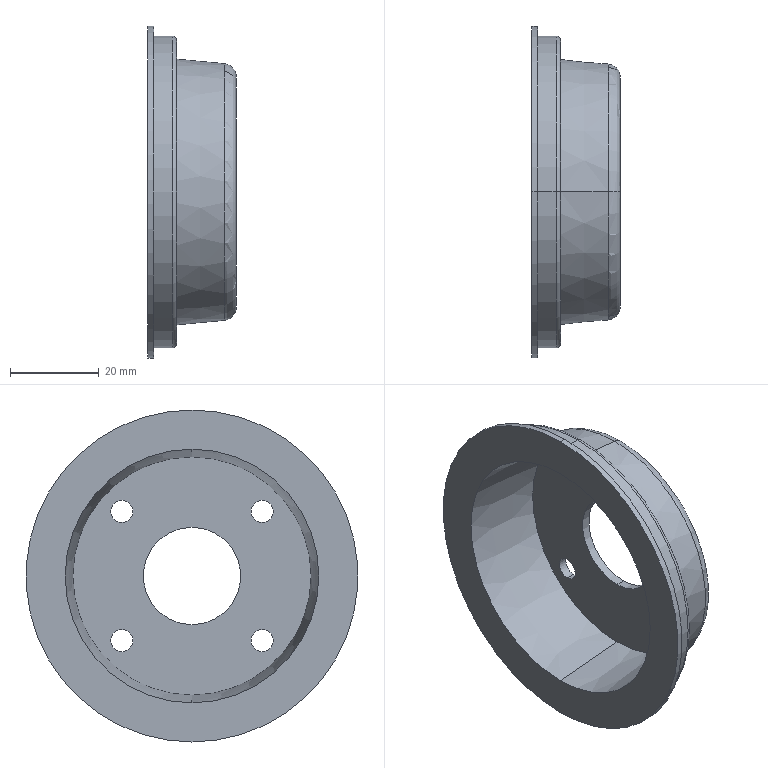Part | SolidWorks | features Fillet 2, ICE 1, Revolution 1 | 1 solid | 27 faces | box 20 x 75 x 75 mm | volume 17771 mm3 | cylinder 14 | plane 5 | torus 4 | cone 4 | commonest cylinder face diameters 5 x8 22 x2 70.467 x2 75 x2
STEP:
#1=CARTESIAN_POINT('',(-54.997,25.565,-34.234));
#2=VERTEX_POINT('',#1);
#3=CARTESIAN_POINT('',(-54.997,25.565,34.234));
#4=VERTEX_POINT('',#3);
#5=CARTESIAN_POINT('',(-54.997,25.565,0.));
#6=DIRECTION('',(1.,0.,0.));
#7=DIRECTION('',(0.,0.,1.));
#8=AXIS2_PLACEMENT_3D('',#5,#6,#7);
#9=CIRCLE('',#8,34.234);
#10=EDGE_CURVE('',#2,#4,#9,.T.);
#11=ORIENTED_EDGE('',*,*,#10,.F.);
#12=CARTESIAN_POINT('',(-55.997,25.565,-35.234));
#13=VERTEX_POINT('',#12);
#14=CARTESIAN_POINT('',(-55.997,25.565,-34.234));
#15=DIRECTION('',(0.,1.,0.));
#16=DIRECTION('',(0.,0.,1.));
#17=AXIS2_PLACEMENT_3D('',#14,#15,#16);
#18=CIRCLE('',#17,1.);
#19=EDGE_CURVE('',#2,#13,#18,.T.);
#20=ORIENTED_EDGE('',*,*,#19,.T.);
#21=CARTESIAN_POINT('',(-55.997,25.565,35.234));
#22=VERTEX_POINT('',#21);
#23=CARTESIAN_POINT('',(-55.997,25.565,0.));
#24=DIRECTION('',(-1.,0.,0.));
#25=DIRECTION('',(0.,0.,1.));
#26=AXIS2_PLACEMENT_3D('',#23,#24,#25);
#27=CIRCLE('',#26,35.234);
#28=EDGE_CURVE('',#22,#13,#27,.T.);
#29=ORIENTED_EDGE('',*,*,#28,.F.);
#30=CARTESIAN_POINT('',(-55.997,25.565,34.234));
#31=DIRECTION('',(0.,-1.,0.));
#32=DIRECTION('',(0.,0.,-1.));
#33=AXIS2_PLACEMENT_3D('',#30,#31,#32);
#34=CIRCLE('',#33,1.);
#35=EDGE_CURVE('',#4,#22,#34,.T.);
#36=ORIENTED_EDGE('',*,*,#35,.F.);
#37=EDGE_LOOP('',(#11,#20,#29,#36));
#38=FACE_OUTER_BOUND('',#37,.T.);
#39=CARTESIAN_POINT('',(-55.997,25.565,0.));
#40=DIRECTION('',(-1.,0.,0.));
#41=DIRECTION('',(0.,0.,1.));
#42=AXIS2_PLACEMENT_3D('',#39,#40,#41);
#43=TOROIDAL_SURFACE('',#42,34.234,1.);
#44=ADVANCED_FACE('',(#38),#43,.T.);
#45=CARTESIAN_POINT('',(-41.497,25.565,-26.009));
#46=VERTEX_POINT('',#45);
#47=CARTESIAN_POINT('',(-41.497,25.565,26.009));
#48=VERTEX_POINT('',#47);
#49=CARTESIAN_POINT('',(-41.497,25.565,0.));
#50=DIRECTION('',(1.,0.,0.));
#51=DIRECTION('',(0.,0.,1.));
#52=AXIS2_PLACEMENT_3D('',#49,#50,#51);
#53=CIRCLE('',#52,26.009);
#54=EDGE_CURVE('',#46,#48,#53,.T.);
#55=ORIENTED_EDGE('',*,*,#54,.F.);
#56=CARTESIAN_POINT('',(-44.211,25.565,-28.995));
#57=VERTEX_POINT('',#56);
#58=CARTESIAN_POINT('',(-44.497,25.565,-26.009));
#59=DIRECTION('',(0.,1.,0.));
#60=DIRECTION('',(0.,0.,1.));
#61=AXIS2_PLACEMENT_3D('',#58,#59,#60);
#62=CIRCLE('',#61,3.);
#63=EDGE_CURVE('',#46,#57,#62,.T.);
#64=ORIENTED_EDGE('',*,*,#63,.T.);
#65=CARTESIAN_POINT('',(-44.211,25.565,28.995));
#66=VERTEX_POINT('',#65);
#67=CARTESIAN_POINT('',(-44.211,25.565,0.));
#68=DIRECTION('',(-1.,0.,0.));
#69=DIRECTION('',(0.,0.,-1.));
#70=AXIS2_PLACEMENT_3D('',#67,#68,#69);
#71=CIRCLE('',#70,28.995);
#72=EDGE_CURVE('',#66,#57,#71,.T.);
#73=ORIENTED_EDGE('',*,*,#72,.F.);
#74=CARTESIAN_POINT('',(-44.497,25.565,26.009));
#75=DIRECTION('',(0.,-1.,0.));
#76=DIRECTION('',(0.,0.,-1.));
#77=AXIS2_PLACEMENT_3D('',#74,#75,#76);
#78=CIRCLE('',#77,3.);
#79=EDGE_CURVE('',#48,#66,#78,.T.);
#80=ORIENTED_EDGE('',*,*,#79,.F.);
#81=EDGE_LOOP('',(#55,#64,#73,#80));
#82=FACE_OUTER_BOUND('',#81,.T.);
#83=CARTESIAN_POINT('',(-44.497,25.565,0.));
#84=DIRECTION('',(-1.,0.,0.));
#85=DIRECTION('',(0.,0.,1.));
#86=AXIS2_PLACEMENT_3D('',#83,#84,#85);
#87=TOROIDAL_SURFACE('',#86,26.009,3.);
#88=ADVANCED_FACE('',(#82),#87,.T.);
#89=CARTESIAN_POINT('',(-43.497,9.71,17.099));
#90=VERTEX_POINT('',#89);
#91=CARTESIAN_POINT('',(-43.497,9.71,12.099));
#92=VERTEX_POINT('',#91);
#93=CARTESIAN_POINT('',(-43.497,9.71,14.599));
#94=DIRECTION('',(1.,0.,0.));
#95=DIRECTION('',(0.,0.,-1.));
#96=AXIS2_PLACEMENT_3D('',#93,#94,#95);
#97=CIRCLE('',#96,2.5);
#98=EDGE_CURVE('',#90,#92,#97,.T.);
#99=ORIENTED_EDGE('',*,*,#98,.F.);
#100=CARTESIAN_POINT('',(-41.497,9.71,17.099));
#101=VERTEX_POINT('',#100);
#102=CARTESIAN_POINT('',(-51.497,9.71,17.099));
#103=DIRECTION('',(1.,0.,0.));
#104=VECTOR('',#103,1000.);
#105=LINE('',#102,#104);
#106=EDGE_CURVE('',#90,#101,#105,.T.);
#107=ORIENTED_EDGE('',*,*,#106,.T.);
#108=CARTESIAN_POINT('',(-41.497,9.71,12.099));
#109=VERTEX_POINT('',#108);
#110=CARTESIAN_POINT('',(-41.497,9.71,14.599));
#111=DIRECTION('',(1.,0.,0.));
#112=DIRECTION('',(0.,0.,1.));
#113=AXIS2_PLACEMENT_3D('',#110,#111,#112);
#114=CIRCLE('',#113,2.5);
#115=EDGE_CURVE('',#101,#109,#114,.T.);
#116=ORIENTED_EDGE('',*,*,#115,.T.);
#117=CARTESIAN_POINT('',(-51.497,9.71,12.099));
#118=DIRECTION('',(1.,0.,0.));
#119=VECTOR('',#118,1000.);
#120=LINE('',#117,#119);
#121=EDGE_CURVE('',#92,#109,#120,.T.);
#122=ORIENTED_EDGE('',*,*,#121,.F.);
#123=EDGE_LOOP('',(#99,#107,#116,#122));
#124=FACE_OUTER_BOUND('',#123,.T.);
#125=CARTESIAN_POINT('',(-51.497,9.71,14.599));
#126=DIRECTION('',(1.,0.,0.));
#127=DIRECTION('',(0.,0.,-1.));
#128=AXIS2_PLACEMENT_3D('',#125,#126,#127);
#129=CYLINDRICAL_SURFACE('',#128,2.5);
#130=ADVANCED_FACE('',(#124),#129,.F.);
#131=CARTESIAN_POINT('',(-43.497,9.71,-12.099));
#132=VERTEX_POINT('',#131);
#133=CARTESIAN_POINT('',(-43.497,9.71,-17.099));
#134=VERTEX_POINT('',#133);
#135=CARTESIAN_POINT('',(-43.497,9.71,-14.599));
#136=DIRECTION('',(1.,0.,0.));
#137=DIRECTION('',(0.,0.,-1.));
#138=AXIS2_PLACEMENT_3D('',#135,#136,#137);
#139=CIRCLE('',#138,2.5);
#140=EDGE_CURVE('',#132,#134,#139,.T.);
#141=ORIENTED_EDGE('',*,*,#140,.F.);
#142=CARTESIAN_POINT('',(-41.497,9.71,-12.099));
#143=VERTEX_POINT('',#142);
#144=CARTESIAN_POINT('',(-51.497,9.71,-12.099));
#145=DIRECTION('',(1.,0.,0.));
#146=VECTOR('',#145,1000.);
#147=LINE('',#144,#146);
#148=EDGE_CURVE('',#132,#143,#147,.T.);
#149=ORIENTED_EDGE('',*,*,#148,.T.);
#150=CARTESIAN_POINT('',(-41.497,9.71,-17.099));
#151=VERTEX_POINT('',#150);
#152=CARTESIAN_POINT('',(-41.497,9.71,-14.599));
#153=DIRECTION('',(1.,0.,0.));
#154=DIRECTION('',(0.,0.,-1.));
#155=AXIS2_PLACEMENT_3D('',#152,#153,#154);
#156=CIRCLE('',#155,2.5);
#157=EDGE_CURVE('',#143,#151,#156,.T.);
#158=ORIENTED_EDGE('',*,*,#157,.T.);
#159=CARTESIAN_POINT('',(-51.497,9.71,-17.099));
#160=DIRECTION('',(1.,0.,0.));
#161=VECTOR('',#160,1000.);
#162=LINE('',#159,#161);
#163=EDGE_CURVE('',#134,#151,#162,.T.);
#164=ORIENTED_EDGE('',*,*,#163,.F.);
#165=EDGE_LOOP('',(#141,#149,#158,#164));
#166=FACE_OUTER_BOUND('',#165,.T.);
#167=CARTESIAN_POINT('',(-51.497,9.71,-14.599));
#168=DIRECTION('',(1.,0.,0.));
#169=DIRECTION('',(0.,0.,-1.));
#170=AXIS2_PLACEMENT_3D('',#167,#168,#169);
#171=CYLINDRICAL_SURFACE('',#170,2.5);
#172=ADVANCED_FACE('',(#166),#171,.F.);
#173=CARTESIAN_POINT('',(-43.497,41.42,-12.099));
#174=VERTEX_POINT('',#173);
#175=CARTESIAN_POINT('',(-43.497,41.42,-17.099));
#176=VERTEX_POINT('',#175);
#177=CARTESIAN_POINT('',(-43.497,41.42,-14.599));
#178=DIRECTION('',(1.,0.,0.));
#179=DIRECTION('',(0.,0.,-1.));
#180=AXIS2_PLACEMENT_3D('',#177,#178,#179);
#181=CIRCLE('',#180,2.5);
#182=EDGE_CURVE('',#174,#176,#181,.T.);
#183=ORIENTED_EDGE('',*,*,#182,.F.);
#184=CARTESIAN_POINT('',(-41.497,41.42,-12.099));
#185=VERTEX_POINT('',#184);
#186=CARTESIAN_POINT('',(-51.497,41.42,-12.099));
#187=DIRECTION('',(1.,0.,0.));
#188=VECTOR('',#187,1000.);
#189=LINE('',#186,#188);
#190=EDGE_CURVE('',#174,#185,#189,.T.);
#191=ORIENTED_EDGE('',*,*,#190,.T.);
#192=CARTESIAN_POINT('',(-41.497,41.42,-17.099));
#193=VERTEX_POINT('',#192);
#194=CARTESIAN_POINT('',(-41.497,41.42,-14.599));
#195=DIRECTION('',(1.,0.,0.));
#196=DIRECTION('',(0.,0.,1.));
#197=AXIS2_PLACEMENT_3D('',#194,#195,#196);
#198=CIRCLE('',#197,2.5);
#199=EDGE_CURVE('',#185,#193,#198,.T.);
#200=ORIENTED_EDGE('',*,*,#199,.T.);
#201=CARTESIAN_POINT('',(-51.497,41.42,-17.099));
#202=DIRECTION('',(1.,0.,0.));
#203=VECTOR('',#202,1000.);
#204=LINE('',#201,#203);
#205=EDGE_CURVE('',#176,#193,#204,.T.);
#206=ORIENTED_EDGE('',*,*,#205,.F.);
#207=EDGE_LOOP('',(#183,#191,#200,#206));
#208=FACE_OUTER_BOUND('',#207,.T.);
#209=CARTESIAN_POINT('',(-51.497,41.42,-14.599));
#210=DIRECTION('',(1.,0.,0.));
#211=DIRECTION('',(0.,0.,-1.));
#212=AXIS2_PLACEMENT_3D('',#209,#210,#211);
#213=CYLINDRICAL_SURFACE('',#212,2.5);
#214=ADVANCED_FACE('',(#208),#213,.F.);
#215=CARTESIAN_POINT('',(-43.497,41.42,17.099));
#216=VERTEX_POINT('',#215);
#217=CARTESIAN_POINT('',(-43.497,41.42,12.099));
#218=VERTEX_POINT('',#217);
#219=CARTESIAN_POINT('',(-43.497,41.42,14.599));
#220=DIRECTION('',(1.,0.,0.));
#221=DIRECTION('',(0.,0.,-1.));
#222=AXIS2_PLACEMENT_3D('',#219,#220,#221);
#223=CIRCLE('',#222,2.5);
#224=EDGE_CURVE('',#216,#218,#223,.T.);
#225=ORIENTED_EDGE('',*,*,#224,.F.);
#226=CARTESIAN_POINT('',(-41.497,41.42,17.099));
#227=VERTEX_POINT('',#226);
#228=CARTESIAN_POINT('',(-51.497,41.42,17.099));
#229=DIRECTION('',(1.,0.,0.));
#230=VECTOR('',#229,1000.);
#231=LINE('',#228,#230);
#232=EDGE_CURVE('',#216,#227,#231,.T.);
#233=ORIENTED_EDGE('',*,*,#232,.T.);
#234=CARTESIAN_POINT('',(-41.497,41.42,12.099));
#235=VERTEX_POINT('',#234);
#236=CARTESIAN_POINT('',(-41.497,41.42,14.599));
#237=DIRECTION('',(1.,0.,0.));
#238=DIRECTION('',(0.,0.,-1.));
#239=AXIS2_PLACEMENT_3D('',#236,#237,#238);
#240=CIRCLE('',#239,2.5);
#241=EDGE_CURVE('',#227,#235,#240,.T.);
#242=ORIENTED_EDGE('',*,*,#241,.T.);
#243=CARTESIAN_POINT('',(-51.497,41.42,12.099));
#244=DIRECTION('',(1.,0.,0.));
#245=VECTOR('',#244,1000.);
#246=LINE('',#243,#245);
#247=EDGE_CURVE('',#218,#235,#246,.T.);
#248=ORIENTED_EDGE('',*,*,#247,.F.);
#249=EDGE_LOOP('',(#225,#233,#242,#248));
#250=FACE_OUTER_BOUND('',#249,.T.);
#251=CARTESIAN_POINT('',(-51.497,41.42,14.599));
#252=DIRECTION('',(1.,0.,0.));
#253=DIRECTION('',(0.,0.,-1.));
#254=AXIS2_PLACEMENT_3D('',#251,#252,#253);
#255=CYLINDRICAL_SURFACE('',#254,2.5);
#256=ADVANCED_FACE('',(#250),#255,.F.);
#257=CARTESIAN_POINT('',(-43.497,25.565,11.));
#258=VERTEX_POINT('',#257);
#259=CARTESIAN_POINT('',(-43.497,25.565,-11.));
#260=VERTEX_POINT('',#259);
#261=CARTESIAN_POINT('',(-43.497,25.565,0.));
#262=DIRECTION('',(1.,0.,0.));
#263=DIRECTION('',(0.,0.,-1.));
#264=AXIS2_PLACEMENT_3D('',#261,#262,#263);
#265=CIRCLE('',#264,11.);
#266=EDGE_CURVE('',#258,#260,#265,.T.);
#267=ORIENTED_EDGE('',*,*,#266,.F.);
#268=CARTESIAN_POINT('',(-41.497,25.565,11.));
#269=VERTEX_POINT('',#268);
#270=CARTESIAN_POINT('',(-51.497,25.565,11.));
#271=DIRECTION('',(1.,0.,0.));
#272=VECTOR('',#271,1000.);
#273=LINE('',#270,#272);
#274=EDGE_CURVE('',#258,#269,#273,.T.);
#275=ORIENTED_EDGE('',*,*,#274,.T.);
#276=CARTESIAN_POINT('',(-41.497,25.565,-11.));
#277=VERTEX_POINT('',#276);
#278=CARTESIAN_POINT('',(-41.497,25.565,0.));
#279=DIRECTION('',(1.,0.,0.));
#280=DIRECTION('',(0.,0.,-1.));
#281=AXIS2_PLACEMENT_3D('',#278,#279,#280);
#282=CIRCLE('',#281,11.);
#283=EDGE_CURVE('',#269,#277,#282,.T.);
#284=ORIENTED_EDGE('',*,*,#283,.T.);
#285=CARTESIAN_POINT('',(-51.497,25.565,-11.));
#286=DIRECTION('',(1.,0.,0.));
#287=VECTOR('',#286,1000.);
#288=LINE('',#285,#287);
#289=EDGE_CURVE('',#260,#277,#288,.T.);
#290=ORIENTED_EDGE('',*,*,#289,.F.);
#291=EDGE_LOOP('',(#267,#275,#284,#290));
#292=FACE_OUTER_BOUND('',#291,.T.);
#293=CARTESIAN_POINT('',(-51.497,25.565,0.));
#294=DIRECTION('',(1.,0.,0.));
#295=DIRECTION('',(0.,0.,-1.));
#296=AXIS2_PLACEMENT_3D('',#293,#294,#295);
#297=CYLINDRICAL_SURFACE('',#296,11.);
#298=ADVANCED_FACE('',(#292),#297,.F.);
#299=ORIENTED_EDGE('',*,*,#72,.T.);
#300=CARTESIAN_POINT('',(-54.997,25.565,-30.029));
#301=VERTEX_POINT('',#300);
#302=CARTESIAN_POINT('',(-41.497,25.565,-28.735));
#303=DIRECTION('',(-0.9954,0.,-0.09539));
#304=VECTOR('',#303,1000.);
#305=LINE('',#302,#304);
#306=EDGE_CURVE('',#57,#301,#305,.T.);
#307=ORIENTED_EDGE('',*,*,#306,.T.);
#308=CARTESIAN_POINT('',(-54.997,25.565,30.029));
#309=VERTEX_POINT('',#308);
#310=CARTESIAN_POINT('',(-54.997,25.565,0.));
#311=DIRECTION('',(-1.,0.,0.));
#312=DIRECTION('',(0.,0.,1.));
#313=AXIS2_PLACEMENT_3D('',#310,#311,#312);
#314=CIRCLE('',#313,30.029);
#315=EDGE_CURVE('',#309,#301,#314,.T.);
#316=ORIENTED_EDGE('',*,*,#315,.F.);
#317=CARTESIAN_POINT('',(-41.497,25.565,28.735));
#318=DIRECTION('',(-0.9954,0.,0.09539));
#319=VECTOR('',#318,1000.);
#320=LINE('',#317,#319);
#321=EDGE_CURVE('',#66,#309,#320,.T.);
#322=ORIENTED_EDGE('',*,*,#321,.F.);
#323=EDGE_LOOP('',(#299,#307,#316,#322));
#324=FACE_OUTER_BOUND('',#323,.T.);
#325=CARTESIAN_POINT('',(-41.497,25.565,0.));
#326=DIRECTION('',(-1.,0.,0.));
#327=DIRECTION('',(0.,0.,1.));
#328=AXIS2_PLACEMENT_3D('',#325,#326,#327);
#329=CONICAL_SURFACE('',#328,28.735,0.09554);
#330=ADVANCED_FACE('',(#324),#329,.T.);
#331=ORIENTED_EDGE('',*,*,#28,.T.);
#332=CARTESIAN_POINT('',(-60.158,25.565,-35.234));
#333=VERTEX_POINT('',#332);
#334=CARTESIAN_POINT('',(-61.497,25.565,-35.234));
#335=DIRECTION('',(-1.,0.,0.));
#336=VECTOR('',#335,1000.);
#337=LINE('',#334,#336);
#338=EDGE_CURVE('',#13,#333,#337,.T.);
#339=ORIENTED_EDGE('',*,*,#338,.T.);
#340=CARTESIAN_POINT('',(-60.158,25.565,35.234));
#341=VERTEX_POINT('',#340);
#342=CARTESIAN_POINT('',(-60.158,25.565,0.));
#343=DIRECTION('',(-1.,0.,0.));
#344=DIRECTION('',(0.,0.,1.));
#345=AXIS2_PLACEMENT_3D('',#342,#343,#344);
#346=CIRCLE('',#345,35.234);
#347=EDGE_CURVE('',#341,#333,#346,.T.);
#348=ORIENTED_EDGE('',*,*,#347,.F.);
#349=CARTESIAN_POINT('',(-61.497,25.565,35.234));
#350=DIRECTION('',(-1.,0.,0.));
#351=VECTOR('',#350,1000.);
#352=LINE('',#349,#351);
#353=EDGE_CURVE('',#22,#341,#352,.T.);
#354=ORIENTED_EDGE('',*,*,#353,.F.);
#355=EDGE_LOOP('',(#331,#339,#348,#354));
#356=FACE_OUTER_BOUND('',#355,.T.);
#357=CARTESIAN_POINT('',(-61.497,25.565,0.));
#358=DIRECTION('',(-1.,0.,0.));
#359=DIRECTION('',(0.,0.,1.));
#360=AXIS2_PLACEMENT_3D('',#357,#358,#359);
#361=CYLINDRICAL_SURFACE('',#360,35.234);
#362=ADVANCED_FACE('',(#356),#361,.T.);
#363=CARTESIAN_POINT('',(-60.158,25.565,37.5));
#364=VERTEX_POINT('',#363);
#365=CARTESIAN_POINT('',(-60.158,25.565,-37.5));
#366=VERTEX_POINT('',#365);
#367=CARTESIAN_POINT('',(-60.158,25.565,0.));
#368=DIRECTION('',(-1.,0.,0.));
#369=DIRECTION('',(0.,0.,1.));
#370=AXIS2_PLACEMENT_3D('',#367,#368,#369);
#371=CIRCLE('',#370,37.5);
#372=EDGE_CURVE('',#364,#366,#371,.T.);
#373=ORIENTED_EDGE('',*,*,#372,.T.);
#374=CARTESIAN_POINT('',(-61.497,25.565,-37.5));
#375=VERTEX_POINT('',#374);
#376=CARTESIAN_POINT('',(-61.497,25.565,-37.5));
#377=DIRECTION('',(-1.,0.,0.));
#378=VECTOR('',#377,1000.);
#379=LINE('',#376,#378);
#380=EDGE_CURVE('',#366,#375,#379,.T.);
#381=ORIENTED_EDGE('',*,*,#380,.T.);
#382=CARTESIAN_POINT('',(-61.497,25.565,37.5));
#383=VERTEX_POINT('',#382);
#384=CARTESIAN_POINT('',(-61.497,25.565,0.));
#385=DIRECTION('',(-1.,0.,0.));
#386=DIRECTION('',(0.,0.,1.));
#387=AXIS2_PLACEMENT_3D('',#384,#385,#386);
#388=CIRCLE('',#387,37.5);
#389=EDGE_CURVE('',#383,#375,#388,.T.);
#390=ORIENTED_EDGE('',*,*,#389,.F.);
#391=CARTESIAN_POINT('',(-61.497,25.565,37.5));
#392=DIRECTION('',(-1.,0.,0.));
#393=VECTOR('',#392,1000.);
#394=LINE('',#391,#393);
#395=EDGE_CURVE('',#364,#383,#394,.T.);
#396=ORIENTED_EDGE('',*,*,#395,.F.);
#397=EDGE_LOOP('',(#373,#381,#390,#396));
#398=FACE_OUTER_BOUND('',#397,.T.);
#399=CARTESIAN_POINT('',(-61.497,25.565,0.));
#400=DIRECTION('',(-1.,0.,0.));
#401=DIRECTION('',(0.,0.,1.));
#402=AXIS2_PLACEMENT_3D('',#399,#400,#401);
#403=CYLINDRICAL_SURFACE('',#402,37.5);
#404=ADVANCED_FACE('',(#398),#403,.T.);
#405=CARTESIAN_POINT('',(-43.497,25.565,-26.918));
#406=VERTEX_POINT('',#405);
#407=CARTESIAN_POINT('',(-43.497,25.565,26.918));
#408=VERTEX_POINT('',#407);
#409=CARTESIAN_POINT('',(-43.497,25.565,0.));
#410=DIRECTION('',(-1.,0.,0.));
#411=DIRECTION('',(0.,0.,1.));
#412=AXIS2_PLACEMENT_3D('',#409,#410,#411);
#413=CIRCLE('',#412,26.918);
#414=EDGE_CURVE('',#406,#408,#413,.T.);
#415=ORIENTED_EDGE('',*,*,#414,.F.);
#416=CARTESIAN_POINT('',(-61.497,25.565,-28.643));
#417=VERTEX_POINT('',#416);
#418=CARTESIAN_POINT('',(-61.497,25.565,-28.643));
#419=DIRECTION('',(-0.9954,0.,-0.09539));
#420=VECTOR('',#419,1000.);
#421=LINE('',#418,#420);
#422=EDGE_CURVE('',#406,#417,#421,.T.);
#423=ORIENTED_EDGE('',*,*,#422,.T.);
#424=CARTESIAN_POINT('',(-61.497,25.565,28.643));
#425=VERTEX_POINT('',#424);
#426=CARTESIAN_POINT('',(-61.497,25.565,0.));
#427=DIRECTION('',(-1.,0.,0.));
#428=DIRECTION('',(0.,0.,1.));
#429=AXIS2_PLACEMENT_3D('',#426,#427,#428);
#430=CIRCLE('',#429,28.643);
#431=EDGE_CURVE('',#417,#425,#430,.T.);
#432=ORIENTED_EDGE('',*,*,#431,.T.);
#433=CARTESIAN_POINT('',(-61.497,25.565,28.643));
#434=DIRECTION('',(-0.9954,0.,0.09539));
#435=VECTOR('',#434,1000.);
#436=LINE('',#433,#435);
#437=EDGE_CURVE('',#408,#425,#436,.T.);
#438=ORIENTED_EDGE('',*,*,#437,.F.);
#439=EDGE_LOOP('',(#415,#423,#432,#438));
#440=FACE_OUTER_BOUND('',#439,.T.);
#441=CARTESIAN_POINT('',(-61.497,25.565,0.));
#442=DIRECTION('',(-1.,0.,0.));
#443=DIRECTION('',(0.,0.,1.));
#444=AXIS2_PLACEMENT_3D('',#441,#442,#443);
#445=CONICAL_SURFACE('',#444,28.643,0.09554);
#446=ADVANCED_FACE('',(#440),#445,.F.);
#447=ORIENTED_EDGE('',*,*,#422,.F.);
#448=CARTESIAN_POINT('',(-43.497,25.565,0.));
#449=DIRECTION('',(-1.,0.,0.));
#450=DIRECTION('',(0.,0.,1.));
#451=AXIS2_PLACEMENT_3D('',#448,#449,#450);
#452=CIRCLE('',#451,26.918);
#453=EDGE_CURVE('',#408,#406,#452,.T.);
#454=ORIENTED_EDGE('',*,*,#453,.F.);
#455=ORIENTED_EDGE('',*,*,#437,.T.);
#456=CARTESIAN_POINT('',(-61.497,25.565,0.));
#457=DIRECTION('',(-1.,0.,0.));
#458=DIRECTION('',(0.,0.,1.));
#459=AXIS2_PLACEMENT_3D('',#456,#457,#458);
#460=CIRCLE('',#459,28.643);
#461=EDGE_CURVE('',#425,#417,#460,.T.);
#462=ORIENTED_EDGE('',*,*,#461,.T.);
#463=EDGE_LOOP('',(#447,#454,#455,#462));
#464=FACE_OUTER_BOUND('',#463,.T.);
#465=CARTESIAN_POINT('',(-61.497,25.565,0.));
#466=DIRECTION('',(-1.,0.,0.));
#467=DIRECTION('',(0.,0.,1.));
#468=AXIS2_PLACEMENT_3D('',#465,#466,#467);
#469=CONICAL_SURFACE('',#468,28.643,0.09554);
#470=ADVANCED_FACE('',(#464),#469,.F.);
#471=ORIENTED_EDGE('',*,*,#461,.F.);
#472=ORIENTED_EDGE('',*,*,#431,.F.);
#473=EDGE_LOOP('',(#471,#472));
#474=FACE_BOUND('',#473,.T.);
#475=ORIENTED_EDGE('',*,*,#389,.T.);
#476=CARTESIAN_POINT('',(-61.497,25.565,0.));
#477=DIRECTION('',(-1.,0.,0.));
#478=DIRECTION('',(0.,0.,1.));
#479=AXIS2_PLACEMENT_3D('',#476,#477,#478);
#480=CIRCLE('',#479,37.5);
#481=EDGE_CURVE('',#375,#383,#480,.T.);
#482=ORIENTED_EDGE('',*,*,#481,.T.);
#483=EDGE_LOOP('',(#475,#482));
#484=FACE_OUTER_BOUND('',#483,.T.);
#485=CARTESIAN_POINT('',(-61.497,54.207,0.));
#486=DIRECTION('',(1.,0.,0.));
#487=DIRECTION('',(0.,0.,-1.));
#488=AXIS2_PLACEMENT_3D('',#485,#486,#487);
#489=PLANE('',#488);
#490=ADVANCED_FACE('',(#474,#484),#489,.F.);
#491=ORIENTED_EDGE('',*,*,#380,.F.);
#492=CARTESIAN_POINT('',(-60.158,25.565,0.));
#493=DIRECTION('',(-1.,0.,0.));
#494=DIRECTION('',(0.,0.,1.));
#495=AXIS2_PLACEMENT_3D('',#492,#493,#494);
#496=CIRCLE('',#495,37.5);
#497=EDGE_CURVE('',#366,#364,#496,.T.);
#498=ORIENTED_EDGE('',*,*,#497,.T.);
#499=ORIENTED_EDGE('',*,*,#395,.T.);
#500=ORIENTED_EDGE('',*,*,#481,.F.);
#501=EDGE_LOOP('',(#491,#498,#499,#500));
#502=FACE_OUTER_BOUND('',#501,.T.);
#503=CARTESIAN_POINT('',(-61.497,25.565,0.));
#504=DIRECTION('',(-1.,0.,0.));
#505=DIRECTION('',(0.,0.,1.));
#506=AXIS2_PLACEMENT_3D('',#503,#504,#505);
#507=CYLINDRICAL_SURFACE('',#506,37.5);
#508=ADVANCED_FACE('',(#502),#507,.T.);
#509=ORIENTED_EDGE('',*,*,#372,.F.);
#510=ORIENTED_EDGE('',*,*,#497,.F.);
#511=EDGE_LOOP('',(#509,#510));
#512=FACE_OUTER_BOUND('',#511,.T.);
#513=ORIENTED_EDGE('',*,*,#347,.T.);
#514=CARTESIAN_POINT('',(-60.158,25.565,0.));
#515=DIRECTION('',(-1.,0.,0.));
#516=DIRECTION('',(0.,0.,1.));
#517=AXIS2_PLACEMENT_3D('',#514,#515,#516);
#518=CIRCLE('',#517,35.234);
#519=EDGE_CURVE('',#333,#341,#518,.T.);
#520=ORIENTED_EDGE('',*,*,#519,.T.);
#521=EDGE_LOOP('',(#513,#520));
#522=FACE_BOUND('',#521,.T.);
#523=CARTESIAN_POINT('',(-60.158,63.065,0.));
#524=DIRECTION('',(-1.,0.,0.));
#525=DIRECTION('',(0.,0.,1.));
#526=AXIS2_PLACEMENT_3D('',#523,#524,#525);
#527=PLANE('',#526);
#528=ADVANCED_FACE('',(#512,#522),#527,.F.);
#529=ORIENTED_EDGE('',*,*,#338,.F.);
#530=CARTESIAN_POINT('',(-55.997,25.565,0.));
#531=DIRECTION('',(-1.,0.,0.));
#532=DIRECTION('',(0.,0.,1.));
#533=AXIS2_PLACEMENT_3D('',#530,#531,#532);
#534=CIRCLE('',#533,35.234);
#535=EDGE_CURVE('',#13,#22,#534,.T.);
#536=ORIENTED_EDGE('',*,*,#535,.T.);
#537=ORIENTED_EDGE('',*,*,#353,.T.);
#538=ORIENTED_EDGE('',*,*,#519,.F.);
#539=EDGE_LOOP('',(#529,#536,#537,#538));
#540=FACE_OUTER_BOUND('',#539,.T.);
#541=CARTESIAN_POINT('',(-61.497,25.565,0.));
#542=DIRECTION('',(-1.,0.,0.));
#543=DIRECTION('',(0.,0.,1.));
#544=AXIS2_PLACEMENT_3D('',#541,#542,#543);
#545=CYLINDRICAL_SURFACE('',#544,35.234);
#546=ADVANCED_FACE('',(#540),#545,.T.);
#547=CARTESIAN_POINT('',(-54.997,25.565,0.));
#548=DIRECTION('',(1.,0.,0.));
#549=DIRECTION('',(0.,0.,1.));
#550=AXIS2_PLACEMENT_3D('',#547,#548,#549);
#551=CIRCLE('',#550,34.234);
#552=EDGE_CURVE('',#4,#2,#551,.T.);
#553=ORIENTED_EDGE('',*,*,#552,.T.);
#554=ORIENTED_EDGE('',*,*,#10,.T.);
#555=EDGE_LOOP('',(#553,#554));
#556=FACE_OUTER_BOUND('',#555,.T.);
#557=ORIENTED_EDGE('',*,*,#315,.T.);
#558=CARTESIAN_POINT('',(-54.997,25.565,0.));
#559=DIRECTION('',(-1.,0.,0.));
#560=DIRECTION('',(0.,0.,1.));
#561=AXIS2_PLACEMENT_3D('',#558,#559,#560);
#562=CIRCLE('',#561,30.029);
#563=EDGE_CURVE('',#301,#309,#562,.T.);
#564=ORIENTED_EDGE('',*,*,#563,.T.);
#565=EDGE_LOOP('',(#557,#564));
#566=FACE_BOUND('',#565,.T.);
#567=CARTESIAN_POINT('',(-54.997,60.798,0.));
#568=DIRECTION('',(-1.,0.,0.));
#569=DIRECTION('',(0.,0.,1.));
#570=AXIS2_PLACEMENT_3D('',#567,#568,#569);
#571=PLANE('',#570);
#572=ADVANCED_FACE('',(#556,#566),#571,.F.);
#573=ORIENTED_EDGE('',*,*,#306,.F.);
#574=CARTESIAN_POINT('',(-44.211,25.565,0.));
#575=DIRECTION('',(-1.,0.,0.));
#576=DIRECTION('',(0.,0.,-1.));
#577=AXIS2_PLACEMENT_3D('',#574,#575,#576);
#578=CIRCLE('',#577,28.995);
#579=EDGE_CURVE('',#57,#66,#578,.T.);
#580=ORIENTED_EDGE('',*,*,#579,.T.);
#581=ORIENTED_EDGE('',*,*,#321,.T.);
#582=ORIENTED_EDGE('',*,*,#563,.F.);
#583=EDGE_LOOP('',(#573,#580,#581,#582));
#584=FACE_OUTER_BOUND('',#583,.T.);
#585=CARTESIAN_POINT('',(-41.497,25.565,0.));
#586=DIRECTION('',(-1.,0.,0.));
#587=DIRECTION('',(0.,0.,1.));
#588=AXIS2_PLACEMENT_3D('',#585,#586,#587);
#589=CONICAL_SURFACE('',#588,28.735,0.09554);
#590=ADVANCED_FACE('',(#584),#589,.T.);
#591=CARTESIAN_POINT('',(-41.497,25.565,0.));
#592=DIRECTION('',(1.,0.,0.));
#593=DIRECTION('',(0.,0.,1.));
#594=AXIS2_PLACEMENT_3D('',#591,#592,#593);
#595=CIRCLE('',#594,26.009);
#596=EDGE_CURVE('',#48,#46,#595,.T.);
#597=ORIENTED_EDGE('',*,*,#596,.T.);
#598=ORIENTED_EDGE('',*,*,#54,.T.);
#599=EDGE_LOOP('',(#597,#598));
#600=FACE_OUTER_BOUND('',#599,.T.);
#601=CARTESIAN_POINT('',(-41.497,9.71,14.599));
#602=DIRECTION('',(1.,0.,0.));
#603=DIRECTION('',(0.,0.,1.));
#604=AXIS2_PLACEMENT_3D('',#601,#602,#603);
#605=CIRCLE('',#604,2.5);
#606=EDGE_CURVE('',#109,#101,#605,.T.);
#607=ORIENTED_EDGE('',*,*,#606,.F.);
#608=ORIENTED_EDGE('',*,*,#115,.F.);
#609=EDGE_LOOP('',(#607,#608));
#610=FACE_BOUND('',#609,.T.);
#611=CARTESIAN_POINT('',(-41.497,9.71,-14.599));
#612=DIRECTION('',(1.,0.,0.));
#613=DIRECTION('',(0.,0.,-1.));
#614=AXIS2_PLACEMENT_3D('',#611,#612,#613);
#615=CIRCLE('',#614,2.5);
#616=EDGE_CURVE('',#151,#143,#615,.T.);
#617=ORIENTED_EDGE('',*,*,#616,.F.);
#618=ORIENTED_EDGE('',*,*,#157,.F.);
#619=EDGE_LOOP('',(#617,#618));
#620=FACE_BOUND('',#619,.T.);
#621=CARTESIAN_POINT('',(-41.497,41.42,-14.599));
#622=DIRECTION('',(1.,0.,0.));
#623=DIRECTION('',(0.,0.,1.));
#624=AXIS2_PLACEMENT_3D('',#621,#622,#623);
#625=CIRCLE('',#624,2.5);
#626=EDGE_CURVE('',#193,#185,#625,.T.);
#627=ORIENTED_EDGE('',*,*,#626,.F.);
#628=ORIENTED_EDGE('',*,*,#199,.F.);
#629=EDGE_LOOP('',(#627,#628));
#630=FACE_BOUND('',#629,.T.);
#631=CARTESIAN_POINT('',(-41.497,41.42,14.599));
#632=DIRECTION('',(1.,0.,0.));
#633=DIRECTION('',(0.,0.,-1.));
#634=AXIS2_PLACEMENT_3D('',#631,#632,#633);
#635=CIRCLE('',#634,2.5);
#636=EDGE_CURVE('',#235,#227,#635,.T.);
#637=ORIENTED_EDGE('',*,*,#636,.F.);
#638=ORIENTED_EDGE('',*,*,#241,.F.);
#639=EDGE_LOOP('',(#637,#638));
#640=FACE_BOUND('',#639,.T.);
#641=CARTESIAN_POINT('',(-41.497,25.565,0.));
#642=DIRECTION('',(1.,0.,0.));
#643=DIRECTION('',(0.,0.,-1.));
#644=AXIS2_PLACEMENT_3D('',#641,#642,#643);
#645=CIRCLE('',#644,11.);
#646=EDGE_CURVE('',#277,#269,#645,.T.);
#647=ORIENTED_EDGE('',*,*,#646,.F.);
#648=ORIENTED_EDGE('',*,*,#283,.F.);
#649=EDGE_LOOP('',(#647,#648));
#650=FACE_BOUND('',#649,.T.);
#651=CARTESIAN_POINT('',(-41.497,54.3,0.));
#652=DIRECTION('',(-1.,0.,0.));
#653=DIRECTION('',(0.,0.,1.));
#654=AXIS2_PLACEMENT_3D('',#651,#652,#653);
#655=PLANE('',#654);
#656=ADVANCED_FACE('',(#600,#610,#620,#630,#640,#650),#655,.F.);
#657=CARTESIAN_POINT('',(-43.497,9.71,14.599));
#658=DIRECTION('',(1.,0.,0.));
#659=DIRECTION('',(0.,0.,-1.));
#660=AXIS2_PLACEMENT_3D('',#657,#658,#659);
#661=CIRCLE('',#660,2.5);
#662=EDGE_CURVE('',#92,#90,#661,.T.);
#663=ORIENTED_EDGE('',*,*,#662,.T.);
#664=ORIENTED_EDGE('',*,*,#98,.T.);
#665=EDGE_LOOP('',(#663,#664));
#666=FACE_BOUND('',#665,.T.);
#667=CARTESIAN_POINT('',(-43.497,9.71,-14.599));
#668=DIRECTION('',(1.,0.,0.));
#669=DIRECTION('',(0.,0.,-1.));
#670=AXIS2_PLACEMENT_3D('',#667,#668,#669);
#671=CIRCLE('',#670,2.5);
#672=EDGE_CURVE('',#134,#132,#671,.T.);
#673=ORIENTED_EDGE('',*,*,#672,.T.);
#674=ORIENTED_EDGE('',*,*,#140,.T.);
#675=EDGE_LOOP('',(#673,#674));
#676=FACE_BOUND('',#675,.T.);
#677=CARTESIAN_POINT('',(-43.497,41.42,-14.599));
#678=DIRECTION('',(1.,0.,0.));
#679=DIRECTION('',(0.,0.,-1.));
#680=AXIS2_PLACEMENT_3D('',#677,#678,#679);
#681=CIRCLE('',#680,2.5);
#682=EDGE_CURVE('',#176,#174,#681,.T.);
#683=ORIENTED_EDGE('',*,*,#682,.T.);
#684=ORIENTED_EDGE('',*,*,#182,.T.);
#685=EDGE_LOOP('',(#683,#684));
#686=FACE_BOUND('',#685,.T.);
#687=CARTESIAN_POINT('',(-43.497,41.42,14.599));
#688=DIRECTION('',(1.,0.,0.));
#689=DIRECTION('',(0.,0.,-1.));
#690=AXIS2_PLACEMENT_3D('',#687,#688,#689);
#691=CIRCLE('',#690,2.5);
#692=EDGE_CURVE('',#218,#216,#691,.T.);
#693=ORIENTED_EDGE('',*,*,#692,.T.);
#694=ORIENTED_EDGE('',*,*,#224,.T.);
#695=EDGE_LOOP('',(#693,#694));
#696=FACE_BOUND('',#695,.T.);
#697=CARTESIAN_POINT('',(-43.497,25.565,0.));
#698=DIRECTION('',(1.,0.,0.));
#699=DIRECTION('',(0.,0.,-1.));
#700=AXIS2_PLACEMENT_3D('',#697,#698,#699);
#701=CIRCLE('',#700,11.);
#702=EDGE_CURVE('',#260,#258,#701,.T.);
#703=ORIENTED_EDGE('',*,*,#702,.T.);
#704=ORIENTED_EDGE('',*,*,#266,.T.);
#705=EDGE_LOOP('',(#703,#704));
#706=FACE_BOUND('',#705,.T.);
#707=ORIENTED_EDGE('',*,*,#453,.T.);
#708=ORIENTED_EDGE('',*,*,#414,.T.);
#709=EDGE_LOOP('',(#707,#708));
#710=FACE_OUTER_BOUND('',#709,.T.);
#711=CARTESIAN_POINT('',(-43.497,52.482,0.));
#712=DIRECTION('',(1.,0.,0.));
#713=DIRECTION('',(0.,0.,-1.));
#714=AXIS2_PLACEMENT_3D('',#711,#712,#713);
#715=PLANE('',#714);
#716=ADVANCED_FACE('',(#666,#676,#686,#696,#706,#710),#715,.F.);
#717=ORIENTED_EDGE('',*,*,#274,.F.);
#718=ORIENTED_EDGE('',*,*,#702,.F.);
#719=ORIENTED_EDGE('',*,*,#289,.T.);
#720=ORIENTED_EDGE('',*,*,#646,.T.);
#721=EDGE_LOOP('',(#717,#718,#719,#720));
#722=FACE_OUTER_BOUND('',#721,.T.);
#723=CARTESIAN_POINT('',(-51.497,25.565,0.));
#724=DIRECTION('',(1.,0.,0.));
#725=DIRECTION('',(0.,0.,-1.));
#726=AXIS2_PLACEMENT_3D('',#723,#724,#725);
#727=CYLINDRICAL_SURFACE('',#726,11.);
#728=ADVANCED_FACE('',(#722),#727,.F.);
#729=ORIENTED_EDGE('',*,*,#232,.F.);
#730=ORIENTED_EDGE('',*,*,#692,.F.);
#731=ORIENTED_EDGE('',*,*,#247,.T.);
#732=ORIENTED_EDGE('',*,*,#636,.T.);
#733=EDGE_LOOP('',(#729,#730,#731,#732));
#734=FACE_OUTER_BOUND('',#733,.T.);
#735=CARTESIAN_POINT('',(-51.497,41.42,14.599));
#736=DIRECTION('',(1.,0.,0.));
#737=DIRECTION('',(0.,0.,-1.));
#738=AXIS2_PLACEMENT_3D('',#735,#736,#737);
#739=CYLINDRICAL_SURFACE('',#738,2.5);
#740=ADVANCED_FACE('',(#734),#739,.F.);
#741=ORIENTED_EDGE('',*,*,#190,.F.);
#742=ORIENTED_EDGE('',*,*,#682,.F.);
#743=ORIENTED_EDGE('',*,*,#205,.T.);
#744=ORIENTED_EDGE('',*,*,#626,.T.);
#745=EDGE_LOOP('',(#741,#742,#743,#744));
#746=FACE_OUTER_BOUND('',#745,.T.);
#747=CARTESIAN_POINT('',(-51.497,41.42,-14.599));
#748=DIRECTION('',(1.,0.,0.));
#749=DIRECTION('',(0.,0.,-1.));
#750=AXIS2_PLACEMENT_3D('',#747,#748,#749);
#751=CYLINDRICAL_SURFACE('',#750,2.5);
#752=ADVANCED_FACE('',(#746),#751,.F.);
#753=ORIENTED_EDGE('',*,*,#148,.F.);
#754=ORIENTED_EDGE('',*,*,#672,.F.);
#755=ORIENTED_EDGE('',*,*,#163,.T.);
#756=ORIENTED_EDGE('',*,*,#616,.T.);
#757=EDGE_LOOP('',(#753,#754,#755,#756));
#758=FACE_OUTER_BOUND('',#757,.T.);
#759=CARTESIAN_POINT('',(-51.497,9.71,-14.599));
#760=DIRECTION('',(1.,0.,0.));
#761=DIRECTION('',(0.,0.,-1.));
#762=AXIS2_PLACEMENT_3D('',#759,#760,#761);
#763=CYLINDRICAL_SURFACE('',#762,2.5);
#764=ADVANCED_FACE('',(#758),#763,.F.);
#765=ORIENTED_EDGE('',*,*,#106,.F.);
#766=ORIENTED_EDGE('',*,*,#662,.F.);
#767=ORIENTED_EDGE('',*,*,#121,.T.);
#768=ORIENTED_EDGE('',*,*,#606,.T.);
#769=EDGE_LOOP('',(#765,#766,#767,#768));
#770=FACE_OUTER_BOUND('',#769,.T.);
#771=CARTESIAN_POINT('',(-51.497,9.71,14.599));
#772=DIRECTION('',(1.,0.,0.));
#773=DIRECTION('',(0.,0.,-1.));
#774=AXIS2_PLACEMENT_3D('',#771,#772,#773);
#775=CYLINDRICAL_SURFACE('',#774,2.5);
#776=ADVANCED_FACE('',(#770),#775,.F.);
#777=ORIENTED_EDGE('',*,*,#63,.F.);
#778=ORIENTED_EDGE('',*,*,#596,.F.);
#779=ORIENTED_EDGE('',*,*,#79,.T.);
#780=ORIENTED_EDGE('',*,*,#579,.F.);
#781=EDGE_LOOP('',(#777,#778,#779,#780));
#782=FACE_OUTER_BOUND('',#781,.T.);
#783=CARTESIAN_POINT('',(-44.497,25.565,0.));
#784=DIRECTION('',(-1.,0.,0.));
#785=DIRECTION('',(0.,0.,1.));
#786=AXIS2_PLACEMENT_3D('',#783,#784,#785);
#787=TOROIDAL_SURFACE('',#786,26.009,3.);
#788=ADVANCED_FACE('',(#782),#787,.T.);
#789=ORIENTED_EDGE('',*,*,#19,.F.);
#790=ORIENTED_EDGE('',*,*,#552,.F.);
#791=ORIENTED_EDGE('',*,*,#35,.T.);
#792=ORIENTED_EDGE('',*,*,#535,.F.);
#793=EDGE_LOOP('',(#789,#790,#791,#792));
#794=FACE_OUTER_BOUND('',#793,.T.);
#795=CARTESIAN_POINT('',(-55.997,25.565,0.));
#796=DIRECTION('',(-1.,0.,0.));
#797=DIRECTION('',(0.,0.,1.));
#798=AXIS2_PLACEMENT_3D('',#795,#796,#797);
#799=TOROIDAL_SURFACE('',#798,34.234,1.);
#800=ADVANCED_FACE('',(#794),#799,.T.);
#801=CLOSED_SHELL('',(#44,#88,#130,#172,#214,#256,#298,#330,#362,#404,#446,#470,#490,#508,#528,#546,#572,#590,#656,#716,#728,#740,#752,#764,#776,#788,#800));
#802=MANIFOLD_SOLID_BREP('',#801);
#803=CARTESIAN_POINT('',(0.,0.,0.));
#804=DIRECTION('',(0.,0.,1.));
#805=DIRECTION('',(1.,0.,0.));
#806=AXIS2_PLACEMENT_3D('',#803,#804,#805);
#807=(LENGTH_UNIT()NAMED_UNIT(*)SI_UNIT(.MILLI.,.METRE.));
#808=UNCERTAINTY_MEASURE_WITH_UNIT(LENGTH_MEASURE(0.00001),#807,'','');
#809=(NAMED_UNIT(*)PLANE_ANGLE_UNIT()SI_UNIT($,.RADIAN.));
#810=(NAMED_UNIT(*)SI_UNIT($,.STERADIAN.)SOLID_ANGLE_UNIT());
#811=(GEOMETRIC_REPRESENTATION_CONTEXT(3)GLOBAL_UNCERTAINTY_ASSIGNED_CONTEXT((#808))GLOBAL_UNIT_ASSIGNED_CONTEXT((#807,#809,#810))REPRESENTATION_CONTEXT('',''));
#812=ADVANCED_BREP_SHAPE_REPRESENTATION('',(#802,#806),#811);